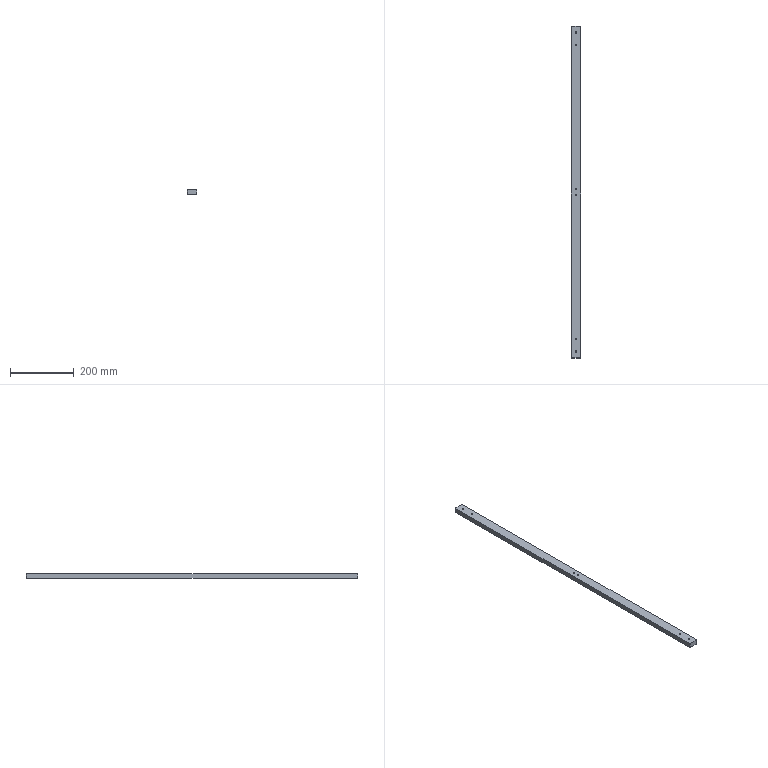Part | SolidWorks | features BaseBody 1 | 1 solid | 22 faces | box 30 x 1038 x 15 mm | volume 465386 mm3 | cylinder 12 | plane 10 | commonest cylinder face diameters 5 x8 4.2 x4
STEP:
#1=CARTESIAN_POINT('',(-2.1,529.,-7.5));
#2=VERTEX_POINT('',#1);
#3=CARTESIAN_POINT('',(2.1,529.,-7.5));
#4=VERTEX_POINT('',#3);
#5=CARTESIAN_POINT('',(0.,529.,-7.5));
#6=DIRECTION('',(0.,0.,1.));
#7=DIRECTION('',(1.,0.,0.));
#8=AXIS2_PLACEMENT_3D('',#5,#6,#7);
#9=CIRCLE('',#8,2.1);
#10=EDGE_CURVE('',#2,#4,#9,.T.);
#11=ORIENTED_EDGE('',*,*,#10,.F.);
#12=CARTESIAN_POINT('',(-2.1,529.,7.5));
#13=VERTEX_POINT('',#12);
#14=CARTESIAN_POINT('',(-2.1,529.,7.5));
#15=DIRECTION('',(0.,0.,1.));
#16=VECTOR('',#15,1000.);
#17=LINE('',#14,#16);
#18=EDGE_CURVE('',#2,#13,#17,.T.);
#19=ORIENTED_EDGE('',*,*,#18,.T.);
#20=CARTESIAN_POINT('',(2.1,529.,7.5));
#21=VERTEX_POINT('',#20);
#22=CARTESIAN_POINT('',(0.,529.,7.5));
#23=DIRECTION('',(0.,0.,1.));
#24=DIRECTION('',(1.,0.,0.));
#25=AXIS2_PLACEMENT_3D('',#22,#23,#24);
#26=CIRCLE('',#25,2.1);
#27=EDGE_CURVE('',#13,#21,#26,.T.);
#28=ORIENTED_EDGE('',*,*,#27,.T.);
#29=CARTESIAN_POINT('',(2.1,529.,7.5));
#30=DIRECTION('',(0.,0.,1.));
#31=VECTOR('',#30,1000.);
#32=LINE('',#29,#31);
#33=EDGE_CURVE('',#4,#21,#32,.T.);
#34=ORIENTED_EDGE('',*,*,#33,.F.);
#35=EDGE_LOOP('',(#11,#19,#28,#34));
#36=FACE_OUTER_BOUND('',#35,.T.);
#37=CARTESIAN_POINT('',(0.,529.,7.5));
#38=DIRECTION('',(0.,0.,1.));
#39=DIRECTION('',(1.,0.,0.));
#40=AXIS2_PLACEMENT_3D('',#37,#38,#39);
#41=CYLINDRICAL_SURFACE('',#40,2.1);
#42=ADVANCED_FACE('',(#36),#41,.F.);
#43=CARTESIAN_POINT('',(-2.1,509.,-7.5));
#44=VERTEX_POINT('',#43);
#45=CARTESIAN_POINT('',(2.1,509.,-7.5));
#46=VERTEX_POINT('',#45);
#47=CARTESIAN_POINT('',(0.,509.,-7.5));
#48=DIRECTION('',(0.,0.,1.));
#49=DIRECTION('',(1.,0.,0.));
#50=AXIS2_PLACEMENT_3D('',#47,#48,#49);
#51=CIRCLE('',#50,2.1);
#52=EDGE_CURVE('',#44,#46,#51,.T.);
#53=ORIENTED_EDGE('',*,*,#52,.F.);
#54=CARTESIAN_POINT('',(-2.1,509.,7.5));
#55=VERTEX_POINT('',#54);
#56=CARTESIAN_POINT('',(-2.1,509.,7.5));
#57=DIRECTION('',(0.,0.,1.));
#58=VECTOR('',#57,1000.);
#59=LINE('',#56,#58);
#60=EDGE_CURVE('',#44,#55,#59,.T.);
#61=ORIENTED_EDGE('',*,*,#60,.T.);
#62=CARTESIAN_POINT('',(2.1,509.,7.5));
#63=VERTEX_POINT('',#62);
#64=CARTESIAN_POINT('',(0.,509.,7.5));
#65=DIRECTION('',(0.,0.,1.));
#66=DIRECTION('',(1.,0.,0.));
#67=AXIS2_PLACEMENT_3D('',#64,#65,#66);
#68=CIRCLE('',#67,2.1);
#69=EDGE_CURVE('',#55,#63,#68,.T.);
#70=ORIENTED_EDGE('',*,*,#69,.T.);
#71=CARTESIAN_POINT('',(2.1,509.,7.5));
#72=DIRECTION('',(0.,0.,1.));
#73=VECTOR('',#72,1000.);
#74=LINE('',#71,#73);
#75=EDGE_CURVE('',#46,#63,#74,.T.);
#76=ORIENTED_EDGE('',*,*,#75,.F.);
#77=EDGE_LOOP('',(#53,#61,#70,#76));
#78=FACE_OUTER_BOUND('',#77,.T.);
#79=CARTESIAN_POINT('',(0.,509.,7.5));
#80=DIRECTION('',(0.,0.,1.));
#81=DIRECTION('',(1.,0.,0.));
#82=AXIS2_PLACEMENT_3D('',#79,#80,#81);
#83=CYLINDRICAL_SURFACE('',#82,2.1);
#84=ADVANCED_FACE('',(#78),#83,.F.);
#85=CARTESIAN_POINT('',(-2.5,1018.,-7.5));
#86=VERTEX_POINT('',#85);
#87=CARTESIAN_POINT('',(2.5,1018.,-7.5));
#88=VERTEX_POINT('',#87);
#89=CARTESIAN_POINT('',(0.,1018.,-7.5));
#90=DIRECTION('',(0.,0.,1.));
#91=DIRECTION('',(1.,0.,0.));
#92=AXIS2_PLACEMENT_3D('',#89,#90,#91);
#93=CIRCLE('',#92,2.5);
#94=EDGE_CURVE('',#86,#88,#93,.T.);
#95=ORIENTED_EDGE('',*,*,#94,.F.);
#96=CARTESIAN_POINT('',(-2.5,1018.,7.5));
#97=VERTEX_POINT('',#96);
#98=CARTESIAN_POINT('',(-2.5,1018.,7.5));
#99=DIRECTION('',(0.,0.,1.));
#100=VECTOR('',#99,1000.);
#101=LINE('',#98,#100);
#102=EDGE_CURVE('',#86,#97,#101,.T.);
#103=ORIENTED_EDGE('',*,*,#102,.T.);
#104=CARTESIAN_POINT('',(2.5,1018.,7.5));
#105=VERTEX_POINT('',#104);
#106=CARTESIAN_POINT('',(0.,1018.,7.5));
#107=DIRECTION('',(0.,0.,1.));
#108=DIRECTION('',(1.,0.,0.));
#109=AXIS2_PLACEMENT_3D('',#106,#107,#108);
#110=CIRCLE('',#109,2.5);
#111=EDGE_CURVE('',#97,#105,#110,.T.);
#112=ORIENTED_EDGE('',*,*,#111,.T.);
#113=CARTESIAN_POINT('',(2.5,1018.,7.5));
#114=DIRECTION('',(0.,0.,1.));
#115=VECTOR('',#114,1000.);
#116=LINE('',#113,#115);
#117=EDGE_CURVE('',#88,#105,#116,.T.);
#118=ORIENTED_EDGE('',*,*,#117,.F.);
#119=EDGE_LOOP('',(#95,#103,#112,#118));
#120=FACE_OUTER_BOUND('',#119,.T.);
#121=CARTESIAN_POINT('',(0.,1018.,7.5));
#122=DIRECTION('',(0.,0.,1.));
#123=DIRECTION('',(1.,0.,0.));
#124=AXIS2_PLACEMENT_3D('',#121,#122,#123);
#125=CYLINDRICAL_SURFACE('',#124,2.5);
#126=ADVANCED_FACE('',(#120),#125,.F.);
#127=CARTESIAN_POINT('',(-2.5,978.,-7.5));
#128=VERTEX_POINT('',#127);
#129=CARTESIAN_POINT('',(2.5,978.,-7.5));
#130=VERTEX_POINT('',#129);
#131=CARTESIAN_POINT('',(0.,978.,-7.5));
#132=DIRECTION('',(0.,0.,1.));
#133=DIRECTION('',(1.,0.,0.));
#134=AXIS2_PLACEMENT_3D('',#131,#132,#133);
#135=CIRCLE('',#134,2.5);
#136=EDGE_CURVE('',#128,#130,#135,.T.);
#137=ORIENTED_EDGE('',*,*,#136,.F.);
#138=CARTESIAN_POINT('',(-2.5,978.,7.5));
#139=VERTEX_POINT('',#138);
#140=CARTESIAN_POINT('',(-2.5,978.,7.5));
#141=DIRECTION('',(0.,0.,1.));
#142=VECTOR('',#141,1000.);
#143=LINE('',#140,#142);
#144=EDGE_CURVE('',#128,#139,#143,.T.);
#145=ORIENTED_EDGE('',*,*,#144,.T.);
#146=CARTESIAN_POINT('',(2.5,978.,7.5));
#147=VERTEX_POINT('',#146);
#148=CARTESIAN_POINT('',(0.,978.,7.5));
#149=DIRECTION('',(0.,0.,1.));
#150=DIRECTION('',(1.,0.,0.));
#151=AXIS2_PLACEMENT_3D('',#148,#149,#150);
#152=CIRCLE('',#151,2.5);
#153=EDGE_CURVE('',#139,#147,#152,.T.);
#154=ORIENTED_EDGE('',*,*,#153,.T.);
#155=CARTESIAN_POINT('',(2.5,978.,7.5));
#156=DIRECTION('',(0.,0.,1.));
#157=VECTOR('',#156,1000.);
#158=LINE('',#155,#157);
#159=EDGE_CURVE('',#130,#147,#158,.T.);
#160=ORIENTED_EDGE('',*,*,#159,.F.);
#161=EDGE_LOOP('',(#137,#145,#154,#160));
#162=FACE_OUTER_BOUND('',#161,.T.);
#163=CARTESIAN_POINT('',(0.,978.,7.5));
#164=DIRECTION('',(0.,0.,1.));
#165=DIRECTION('',(1.,0.,0.));
#166=AXIS2_PLACEMENT_3D('',#163,#164,#165);
#167=CYLINDRICAL_SURFACE('',#166,2.5);
#168=ADVANCED_FACE('',(#162),#167,.F.);
#169=CARTESIAN_POINT('',(-2.5,20.,-7.5));
#170=VERTEX_POINT('',#169);
#171=CARTESIAN_POINT('',(2.5,20.,-7.5));
#172=VERTEX_POINT('',#171);
#173=CARTESIAN_POINT('',(0.,20.,-7.5));
#174=DIRECTION('',(0.,0.,1.));
#175=DIRECTION('',(1.,0.,0.));
#176=AXIS2_PLACEMENT_3D('',#173,#174,#175);
#177=CIRCLE('',#176,2.5);
#178=EDGE_CURVE('',#170,#172,#177,.T.);
#179=ORIENTED_EDGE('',*,*,#178,.F.);
#180=CARTESIAN_POINT('',(-2.5,20.,7.5));
#181=VERTEX_POINT('',#180);
#182=CARTESIAN_POINT('',(-2.5,20.,7.5));
#183=DIRECTION('',(0.,0.,1.));
#184=VECTOR('',#183,1000.);
#185=LINE('',#182,#184);
#186=EDGE_CURVE('',#170,#181,#185,.T.);
#187=ORIENTED_EDGE('',*,*,#186,.T.);
#188=CARTESIAN_POINT('',(2.5,20.,7.5));
#189=VERTEX_POINT('',#188);
#190=CARTESIAN_POINT('',(0.,20.,7.5));
#191=DIRECTION('',(0.,0.,1.));
#192=DIRECTION('',(1.,0.,0.));
#193=AXIS2_PLACEMENT_3D('',#190,#191,#192);
#194=CIRCLE('',#193,2.5);
#195=EDGE_CURVE('',#181,#189,#194,.T.);
#196=ORIENTED_EDGE('',*,*,#195,.T.);
#197=CARTESIAN_POINT('',(2.5,20.,7.5));
#198=DIRECTION('',(0.,0.,1.));
#199=VECTOR('',#198,1000.);
#200=LINE('',#197,#199);
#201=EDGE_CURVE('',#172,#189,#200,.T.);
#202=ORIENTED_EDGE('',*,*,#201,.F.);
#203=EDGE_LOOP('',(#179,#187,#196,#202));
#204=FACE_OUTER_BOUND('',#203,.T.);
#205=CARTESIAN_POINT('',(0.,20.,7.5));
#206=DIRECTION('',(0.,0.,1.));
#207=DIRECTION('',(1.,0.,0.));
#208=AXIS2_PLACEMENT_3D('',#205,#206,#207);
#209=CYLINDRICAL_SURFACE('',#208,2.5);
#210=ADVANCED_FACE('',(#204),#209,.F.);
#211=CARTESIAN_POINT('',(-2.5,60.,-7.5));
#212=VERTEX_POINT('',#211);
#213=CARTESIAN_POINT('',(2.5,60.,-7.5));
#214=VERTEX_POINT('',#213);
#215=CARTESIAN_POINT('',(0.,60.,-7.5));
#216=DIRECTION('',(0.,0.,1.));
#217=DIRECTION('',(1.,0.,0.));
#218=AXIS2_PLACEMENT_3D('',#215,#216,#217);
#219=CIRCLE('',#218,2.5);
#220=EDGE_CURVE('',#212,#214,#219,.T.);
#221=ORIENTED_EDGE('',*,*,#220,.F.);
#222=CARTESIAN_POINT('',(-2.5,60.,7.5));
#223=VERTEX_POINT('',#222);
#224=CARTESIAN_POINT('',(-2.5,60.,7.5));
#225=DIRECTION('',(0.,0.,1.));
#226=VECTOR('',#225,1000.);
#227=LINE('',#224,#226);
#228=EDGE_CURVE('',#212,#223,#227,.T.);
#229=ORIENTED_EDGE('',*,*,#228,.T.);
#230=CARTESIAN_POINT('',(2.5,60.,7.5));
#231=VERTEX_POINT('',#230);
#232=CARTESIAN_POINT('',(0.,60.,7.5));
#233=DIRECTION('',(0.,0.,1.));
#234=DIRECTION('',(1.,0.,0.));
#235=AXIS2_PLACEMENT_3D('',#232,#233,#234);
#236=CIRCLE('',#235,2.5);
#237=EDGE_CURVE('',#223,#231,#236,.T.);
#238=ORIENTED_EDGE('',*,*,#237,.T.);
#239=CARTESIAN_POINT('',(2.5,60.,7.5));
#240=DIRECTION('',(0.,0.,1.));
#241=VECTOR('',#240,1000.);
#242=LINE('',#239,#241);
#243=EDGE_CURVE('',#214,#231,#242,.T.);
#244=ORIENTED_EDGE('',*,*,#243,.F.);
#245=EDGE_LOOP('',(#221,#229,#238,#244));
#246=FACE_OUTER_BOUND('',#245,.T.);
#247=CARTESIAN_POINT('',(0.,60.,7.5));
#248=DIRECTION('',(0.,0.,1.));
#249=DIRECTION('',(1.,0.,0.));
#250=AXIS2_PLACEMENT_3D('',#247,#248,#249);
#251=CYLINDRICAL_SURFACE('',#250,2.5);
#252=ADVANCED_FACE('',(#246),#251,.F.);
#253=CARTESIAN_POINT('',(-15.,1036.,-7.5));
#254=VERTEX_POINT('',#253);
#255=CARTESIAN_POINT('',(-13.,1038.,-7.5));
#256=VERTEX_POINT('',#255);
#257=CARTESIAN_POINT('',(-13.,1038.,-7.5));
#258=DIRECTION('',(0.7071,0.7071,0.));
#259=VECTOR('',#258,1000.);
#260=LINE('',#257,#259);
#261=EDGE_CURVE('',#254,#256,#260,.T.);
#262=ORIENTED_EDGE('',*,*,#261,.F.);
#263=CARTESIAN_POINT('',(-15.,1036.,7.5));
#264=VERTEX_POINT('',#263);
#265=CARTESIAN_POINT('',(-15.,1036.,-7.5));
#266=DIRECTION('',(0.,0.,-1.));
#267=VECTOR('',#266,1000.);
#268=LINE('',#265,#267);
#269=EDGE_CURVE('',#264,#254,#268,.T.);
#270=ORIENTED_EDGE('',*,*,#269,.F.);
#271=CARTESIAN_POINT('',(-13.,1038.,7.5));
#272=VERTEX_POINT('',#271);
#273=CARTESIAN_POINT('',(-13.,1038.,7.5));
#274=DIRECTION('',(-0.7071,-0.7071,0.));
#275=VECTOR('',#274,1000.);
#276=LINE('',#273,#275);
#277=EDGE_CURVE('',#272,#264,#276,.T.);
#278=ORIENTED_EDGE('',*,*,#277,.F.);
#279=CARTESIAN_POINT('',(-13.,1038.,7.5));
#280=DIRECTION('',(0.,0.,1.));
#281=VECTOR('',#280,1000.);
#282=LINE('',#279,#281);
#283=EDGE_CURVE('',#256,#272,#282,.T.);
#284=ORIENTED_EDGE('',*,*,#283,.F.);
#285=EDGE_LOOP('',(#262,#270,#278,#284));
#286=FACE_OUTER_BOUND('',#285,.T.);
#287=CARTESIAN_POINT('',(-13.,1038.,0.));
#288=DIRECTION('',(-0.7071,0.7071,0.));
#289=DIRECTION('',(0.,0.,1.));
#290=AXIS2_PLACEMENT_3D('',#287,#288,#289);
#291=PLANE('',#290);
#292=ADVANCED_FACE('',(#286),#291,.T.);
#293=CARTESIAN_POINT('',(15.,1036.,7.5));
#294=VERTEX_POINT('',#293);
#295=CARTESIAN_POINT('',(13.,1038.,7.5));
#296=VERTEX_POINT('',#295);
#297=CARTESIAN_POINT('',(13.,1038.,7.5));
#298=DIRECTION('',(-0.7071,0.7071,0.));
#299=VECTOR('',#298,1000.);
#300=LINE('',#297,#299);
#301=EDGE_CURVE('',#294,#296,#300,.T.);
#302=ORIENTED_EDGE('',*,*,#301,.F.);
#303=CARTESIAN_POINT('',(15.,1036.,-7.5));
#304=VERTEX_POINT('',#303);
#305=CARTESIAN_POINT('',(15.,1036.,7.5));
#306=DIRECTION('',(0.,0.,1.));
#307=VECTOR('',#306,1000.);
#308=LINE('',#305,#307);
#309=EDGE_CURVE('',#304,#294,#308,.T.);
#310=ORIENTED_EDGE('',*,*,#309,.F.);
#311=CARTESIAN_POINT('',(13.,1038.,-7.5));
#312=VERTEX_POINT('',#311);
#313=CARTESIAN_POINT('',(13.,1038.,-7.5));
#314=DIRECTION('',(0.7071,-0.7071,0.));
#315=VECTOR('',#314,1000.);
#316=LINE('',#313,#315);
#317=EDGE_CURVE('',#312,#304,#316,.T.);
#318=ORIENTED_EDGE('',*,*,#317,.F.);
#319=CARTESIAN_POINT('',(13.,1038.,-7.5));
#320=DIRECTION('',(0.,0.,-1.));
#321=VECTOR('',#320,1000.);
#322=LINE('',#319,#321);
#323=EDGE_CURVE('',#296,#312,#322,.T.);
#324=ORIENTED_EDGE('',*,*,#323,.F.);
#325=EDGE_LOOP('',(#302,#310,#318,#324));
#326=FACE_OUTER_BOUND('',#325,.T.);
#327=CARTESIAN_POINT('',(13.,1038.,0.));
#328=DIRECTION('',(0.7071,0.7071,0.));
#329=DIRECTION('',(0.,0.,-1.));
#330=AXIS2_PLACEMENT_3D('',#327,#328,#329);
#331=PLANE('',#330);
#332=ADVANCED_FACE('',(#326),#331,.T.);
#333=CARTESIAN_POINT('',(-13.,0.,-7.5));
#334=VERTEX_POINT('',#333);
#335=CARTESIAN_POINT('',(-15.,2.,-7.5));
#336=VERTEX_POINT('',#335);
#337=CARTESIAN_POINT('',(-15.,2.,-7.5));
#338=DIRECTION('',(-0.7071,0.7071,0.));
#339=VECTOR('',#338,1000.);
#340=LINE('',#337,#339);
#341=EDGE_CURVE('',#334,#336,#340,.T.);
#342=ORIENTED_EDGE('',*,*,#341,.F.);
#343=CARTESIAN_POINT('',(-13.,0.,7.5));
#344=VERTEX_POINT('',#343);
#345=CARTESIAN_POINT('',(-13.,0.,0.));
#346=DIRECTION('',(0.,0.,-1.));
#347=VECTOR('',#346,1000.);
#348=LINE('',#345,#347);
#349=EDGE_CURVE('',#344,#334,#348,.T.);
#350=ORIENTED_EDGE('',*,*,#349,.F.);
#351=CARTESIAN_POINT('',(-15.,2.,7.5));
#352=VERTEX_POINT('',#351);
#353=CARTESIAN_POINT('',(-15.,2.,7.5));
#354=DIRECTION('',(0.7071,-0.7071,0.));
#355=VECTOR('',#354,1000.);
#356=LINE('',#353,#355);
#357=EDGE_CURVE('',#352,#344,#356,.T.);
#358=ORIENTED_EDGE('',*,*,#357,.F.);
#359=CARTESIAN_POINT('',(-15.,2.,-7.5));
#360=DIRECTION('',(0.,0.,1.));
#361=VECTOR('',#360,1000.);
#362=LINE('',#359,#361);
#363=EDGE_CURVE('',#336,#352,#362,.T.);
#364=ORIENTED_EDGE('',*,*,#363,.F.);
#365=EDGE_LOOP('',(#342,#350,#358,#364));
#366=FACE_OUTER_BOUND('',#365,.T.);
#367=CARTESIAN_POINT('',(-15.,2.,-7.5));
#368=DIRECTION('',(0.7071,0.7071,0.));
#369=DIRECTION('',(0.,0.,-1.));
#370=AXIS2_PLACEMENT_3D('',#367,#368,#369);
#371=PLANE('',#370);
#372=ADVANCED_FACE('',(#366),#371,.F.);
#373=CARTESIAN_POINT('',(13.,0.,7.5));
#374=VERTEX_POINT('',#373);
#375=CARTESIAN_POINT('',(15.,2.,7.5));
#376=VERTEX_POINT('',#375);
#377=CARTESIAN_POINT('',(15.,2.,7.5));
#378=DIRECTION('',(0.7071,0.7071,0.));
#379=VECTOR('',#378,1000.);
#380=LINE('',#377,#379);
#381=EDGE_CURVE('',#374,#376,#380,.T.);
#382=ORIENTED_EDGE('',*,*,#381,.F.);
#383=CARTESIAN_POINT('',(13.,0.,-7.5));
#384=VERTEX_POINT('',#383);
#385=CARTESIAN_POINT('',(13.,0.,0.));
#386=DIRECTION('',(0.,0.,1.));
#387=VECTOR('',#386,1000.);
#388=LINE('',#385,#387);
#389=EDGE_CURVE('',#384,#374,#388,.T.);
#390=ORIENTED_EDGE('',*,*,#389,.F.);
#391=CARTESIAN_POINT('',(15.,2.,-7.5));
#392=VERTEX_POINT('',#391);
#393=CARTESIAN_POINT('',(15.,2.,-7.5));
#394=DIRECTION('',(-0.7071,-0.7071,0.));
#395=VECTOR('',#394,1000.);
#396=LINE('',#393,#395);
#397=EDGE_CURVE('',#392,#384,#396,.T.);
#398=ORIENTED_EDGE('',*,*,#397,.F.);
#399=CARTESIAN_POINT('',(15.,2.,-7.5));
#400=DIRECTION('',(0.,0.,-1.));
#401=VECTOR('',#400,1000.);
#402=LINE('',#399,#401);
#403=EDGE_CURVE('',#376,#392,#402,.T.);
#404=ORIENTED_EDGE('',*,*,#403,.F.);
#405=EDGE_LOOP('',(#382,#390,#398,#404));
#406=FACE_OUTER_BOUND('',#405,.T.);
#407=CARTESIAN_POINT('',(15.,2.,-7.5));
#408=DIRECTION('',(-0.7071,0.7071,0.));
#409=DIRECTION('',(0.,0.,1.));
#410=AXIS2_PLACEMENT_3D('',#407,#408,#409);
#411=PLANE('',#410);
#412=ADVANCED_FACE('',(#406),#411,.F.);
#413=CARTESIAN_POINT('',(-15.,0.,-7.5));
#414=DIRECTION('',(-1.,0.,0.));
#415=VECTOR('',#414,1000.);
#416=LINE('',#413,#415);
#417=EDGE_CURVE('',#384,#334,#416,.T.);
#418=ORIENTED_EDGE('',*,*,#417,.F.);
#419=ORIENTED_EDGE('',*,*,#389,.T.);
#420=CARTESIAN_POINT('',(-15.,0.,7.5));
#421=DIRECTION('',(1.,0.,0.));
#422=VECTOR('',#421,1000.);
#423=LINE('',#420,#422);
#424=EDGE_CURVE('',#344,#374,#423,.T.);
#425=ORIENTED_EDGE('',*,*,#424,.F.);
#426=ORIENTED_EDGE('',*,*,#349,.T.);
#427=EDGE_LOOP('',(#418,#419,#425,#426));
#428=FACE_OUTER_BOUND('',#427,.T.);
#429=CARTESIAN_POINT('',(0.,0.,0.));
#430=DIRECTION('',(0.,1.,0.));
#431=DIRECTION('',(1.,0.,0.));
#432=AXIS2_PLACEMENT_3D('',#429,#430,#431);
#433=PLANE('',#432);
#434=ADVANCED_FACE('',(#428),#433,.F.);
#435=CARTESIAN_POINT('',(-15.,1038.,7.5));
#436=DIRECTION('',(1.,0.,0.));
#437=VECTOR('',#436,1000.);
#438=LINE('',#435,#437);
#439=EDGE_CURVE('',#272,#296,#438,.T.);
#440=ORIENTED_EDGE('',*,*,#439,.T.);
#441=ORIENTED_EDGE('',*,*,#323,.T.);
#442=CARTESIAN_POINT('',(-15.,1038.,-7.5));
#443=DIRECTION('',(-1.,0.,0.));
#444=VECTOR('',#443,1000.);
#445=LINE('',#442,#444);
#446=EDGE_CURVE('',#312,#256,#445,.T.);
#447=ORIENTED_EDGE('',*,*,#446,.T.);
#448=ORIENTED_EDGE('',*,*,#283,.T.);
#449=EDGE_LOOP('',(#440,#441,#447,#448));
#450=FACE_OUTER_BOUND('',#449,.T.);
#451=CARTESIAN_POINT('',(0.,1038.,0.));
#452=DIRECTION('',(0.,1.,0.));
#453=DIRECTION('',(1.,0.,0.));
#454=AXIS2_PLACEMENT_3D('',#451,#452,#453);
#455=PLANE('',#454);
#456=ADVANCED_FACE('',(#450),#455,.T.);
#457=CARTESIAN_POINT('',(0.,60.,7.5));
#458=DIRECTION('',(0.,0.,1.));
#459=DIRECTION('',(1.,0.,0.));
#460=AXIS2_PLACEMENT_3D('',#457,#458,#459);
#461=CIRCLE('',#460,2.5);
#462=EDGE_CURVE('',#231,#223,#461,.T.);
#463=ORIENTED_EDGE('',*,*,#462,.F.);
#464=ORIENTED_EDGE('',*,*,#237,.F.);
#465=EDGE_LOOP('',(#463,#464));
#466=FACE_BOUND('',#465,.T.);
#467=CARTESIAN_POINT('',(0.,20.,7.5));
#468=DIRECTION('',(0.,0.,1.));
#469=DIRECTION('',(1.,0.,0.));
#470=AXIS2_PLACEMENT_3D('',#467,#468,#469);
#471=CIRCLE('',#470,2.5);
#472=EDGE_CURVE('',#189,#181,#471,.T.);
#473=ORIENTED_EDGE('',*,*,#472,.F.);
#474=ORIENTED_EDGE('',*,*,#195,.F.);
#475=EDGE_LOOP('',(#473,#474));
#476=FACE_BOUND('',#475,.T.);
#477=CARTESIAN_POINT('',(0.,978.,7.5));
#478=DIRECTION('',(0.,0.,1.));
#479=DIRECTION('',(1.,0.,0.));
#480=AXIS2_PLACEMENT_3D('',#477,#478,#479);
#481=CIRCLE('',#480,2.5);
#482=EDGE_CURVE('',#147,#139,#481,.T.);
#483=ORIENTED_EDGE('',*,*,#482,.F.);
#484=ORIENTED_EDGE('',*,*,#153,.F.);
#485=EDGE_LOOP('',(#483,#484));
#486=FACE_BOUND('',#485,.T.);
#487=CARTESIAN_POINT('',(0.,1018.,7.5));
#488=DIRECTION('',(0.,0.,1.));
#489=DIRECTION('',(1.,0.,0.));
#490=AXIS2_PLACEMENT_3D('',#487,#488,#489);
#491=CIRCLE('',#490,2.5);
#492=EDGE_CURVE('',#105,#97,#491,.T.);
#493=ORIENTED_EDGE('',*,*,#492,.F.);
#494=ORIENTED_EDGE('',*,*,#111,.F.);
#495=EDGE_LOOP('',(#493,#494));
#496=FACE_BOUND('',#495,.T.);
#497=CARTESIAN_POINT('',(0.,509.,7.5));
#498=DIRECTION('',(0.,0.,1.));
#499=DIRECTION('',(1.,0.,0.));
#500=AXIS2_PLACEMENT_3D('',#497,#498,#499);
#501=CIRCLE('',#500,2.1);
#502=EDGE_CURVE('',#63,#55,#501,.T.);
#503=ORIENTED_EDGE('',*,*,#502,.F.);
#504=ORIENTED_EDGE('',*,*,#69,.F.);
#505=EDGE_LOOP('',(#503,#504));
#506=FACE_BOUND('',#505,.T.);
#507=CARTESIAN_POINT('',(0.,529.,7.5));
#508=DIRECTION('',(0.,0.,1.));
#509=DIRECTION('',(1.,0.,0.));
#510=AXIS2_PLACEMENT_3D('',#507,#508,#509);
#511=CIRCLE('',#510,2.1);
#512=EDGE_CURVE('',#21,#13,#511,.T.);
#513=ORIENTED_EDGE('',*,*,#512,.F.);
#514=ORIENTED_EDGE('',*,*,#27,.F.);
#515=EDGE_LOOP('',(#513,#514));
#516=FACE_BOUND('',#515,.T.);
#517=ORIENTED_EDGE('',*,*,#424,.T.);
#518=ORIENTED_EDGE('',*,*,#381,.T.);
#519=CARTESIAN_POINT('',(15.,1038.,7.5));
#520=DIRECTION('',(0.,-1.,0.));
#521=VECTOR('',#520,1000.);
#522=LINE('',#519,#521);
#523=EDGE_CURVE('',#294,#376,#522,.T.);
#524=ORIENTED_EDGE('',*,*,#523,.F.);
#525=ORIENTED_EDGE('',*,*,#301,.T.);
#526=ORIENTED_EDGE('',*,*,#439,.F.);
#527=ORIENTED_EDGE('',*,*,#277,.T.);
#528=CARTESIAN_POINT('',(-15.,1038.,7.5));
#529=DIRECTION('',(0.,-1.,0.));
#530=VECTOR('',#529,1000.);
#531=LINE('',#528,#530);
#532=EDGE_CURVE('',#264,#352,#531,.T.);
#533=ORIENTED_EDGE('',*,*,#532,.T.);
#534=ORIENTED_EDGE('',*,*,#357,.T.);
#535=EDGE_LOOP('',(#517,#518,#524,#525,#526,#527,#533,#534));
#536=FACE_OUTER_BOUND('',#535,.T.);
#537=CARTESIAN_POINT('',(-15.,1038.,7.5));
#538=DIRECTION('',(0.,0.,-1.));
#539=DIRECTION('',(0.,-1.,0.));
#540=AXIS2_PLACEMENT_3D('',#537,#538,#539);
#541=PLANE('',#540);
#542=ADVANCED_FACE('',(#466,#476,#486,#496,#506,#516,#536),#541,.F.);
#543=CARTESIAN_POINT('',(-15.,1038.,-7.5));
#544=DIRECTION('',(0.,-1.,0.));
#545=VECTOR('',#544,1000.);
#546=LINE('',#543,#545);
#547=EDGE_CURVE('',#254,#336,#546,.T.);
#548=ORIENTED_EDGE('',*,*,#547,.T.);
#549=ORIENTED_EDGE('',*,*,#363,.T.);
#550=ORIENTED_EDGE('',*,*,#532,.F.);
#551=ORIENTED_EDGE('',*,*,#269,.T.);
#552=EDGE_LOOP('',(#548,#549,#550,#551));
#553=FACE_OUTER_BOUND('',#552,.T.);
#554=CARTESIAN_POINT('',(-15.,1038.,-7.5));
#555=DIRECTION('',(1.,0.,0.));
#556=DIRECTION('',(0.,0.,-1.));
#557=AXIS2_PLACEMENT_3D('',#554,#555,#556);
#558=PLANE('',#557);
#559=ADVANCED_FACE('',(#553),#558,.F.);
#560=CARTESIAN_POINT('',(0.,60.,-7.5));
#561=DIRECTION('',(0.,0.,1.));
#562=DIRECTION('',(1.,0.,0.));
#563=AXIS2_PLACEMENT_3D('',#560,#561,#562);
#564=CIRCLE('',#563,2.5);
#565=EDGE_CURVE('',#214,#212,#564,.T.);
#566=ORIENTED_EDGE('',*,*,#565,.T.);
#567=ORIENTED_EDGE('',*,*,#220,.T.);
#568=EDGE_LOOP('',(#566,#567));
#569=FACE_BOUND('',#568,.T.);
#570=CARTESIAN_POINT('',(0.,20.,-7.5));
#571=DIRECTION('',(0.,0.,1.));
#572=DIRECTION('',(1.,0.,0.));
#573=AXIS2_PLACEMENT_3D('',#570,#571,#572);
#574=CIRCLE('',#573,2.5);
#575=EDGE_CURVE('',#172,#170,#574,.T.);
#576=ORIENTED_EDGE('',*,*,#575,.T.);
#577=ORIENTED_EDGE('',*,*,#178,.T.);
#578=EDGE_LOOP('',(#576,#577));
#579=FACE_BOUND('',#578,.T.);
#580=CARTESIAN_POINT('',(0.,978.,-7.5));
#581=DIRECTION('',(0.,0.,1.));
#582=DIRECTION('',(1.,0.,0.));
#583=AXIS2_PLACEMENT_3D('',#580,#581,#582);
#584=CIRCLE('',#583,2.5);
#585=EDGE_CURVE('',#130,#128,#584,.T.);
#586=ORIENTED_EDGE('',*,*,#585,.T.);
#587=ORIENTED_EDGE('',*,*,#136,.T.);
#588=EDGE_LOOP('',(#586,#587));
#589=FACE_BOUND('',#588,.T.);
#590=CARTESIAN_POINT('',(0.,1018.,-7.5));
#591=DIRECTION('',(0.,0.,1.));
#592=DIRECTION('',(1.,0.,0.));
#593=AXIS2_PLACEMENT_3D('',#590,#591,#592);
#594=CIRCLE('',#593,2.5);
#595=EDGE_CURVE('',#88,#86,#594,.T.);
#596=ORIENTED_EDGE('',*,*,#595,.T.);
#597=ORIENTED_EDGE('',*,*,#94,.T.);
#598=EDGE_LOOP('',(#596,#597));
#599=FACE_BOUND('',#598,.T.);
#600=CARTESIAN_POINT('',(0.,509.,-7.5));
#601=DIRECTION('',(0.,0.,1.));
#602=DIRECTION('',(1.,0.,0.));
#603=AXIS2_PLACEMENT_3D('',#600,#601,#602);
#604=CIRCLE('',#603,2.1);
#605=EDGE_CURVE('',#46,#44,#604,.T.);
#606=ORIENTED_EDGE('',*,*,#605,.T.);
#607=ORIENTED_EDGE('',*,*,#52,.T.);
#608=EDGE_LOOP('',(#606,#607));
#609=FACE_BOUND('',#608,.T.);
#610=CARTESIAN_POINT('',(0.,529.,-7.5));
#611=DIRECTION('',(0.,0.,1.));
#612=DIRECTION('',(1.,0.,0.));
#613=AXIS2_PLACEMENT_3D('',#610,#611,#612);
#614=CIRCLE('',#613,2.1);
#615=EDGE_CURVE('',#4,#2,#614,.T.);
#616=ORIENTED_EDGE('',*,*,#615,.T.);
#617=ORIENTED_EDGE('',*,*,#10,.T.);
#618=EDGE_LOOP('',(#616,#617));
#619=FACE_BOUND('',#618,.T.);
#620=CARTESIAN_POINT('',(15.,1038.,-7.5));
#621=DIRECTION('',(0.,-1.,0.));
#622=VECTOR('',#621,1000.);
#623=LINE('',#620,#622);
#624=EDGE_CURVE('',#304,#392,#623,.T.);
#625=ORIENTED_EDGE('',*,*,#624,.T.);
#626=ORIENTED_EDGE('',*,*,#397,.T.);
#627=ORIENTED_EDGE('',*,*,#417,.T.);
#628=ORIENTED_EDGE('',*,*,#341,.T.);
#629=ORIENTED_EDGE('',*,*,#547,.F.);
#630=ORIENTED_EDGE('',*,*,#261,.T.);
#631=ORIENTED_EDGE('',*,*,#446,.F.);
#632=ORIENTED_EDGE('',*,*,#317,.T.);
#633=EDGE_LOOP('',(#625,#626,#627,#628,#629,#630,#631,#632));
#634=FACE_OUTER_BOUND('',#633,.T.);
#635=CARTESIAN_POINT('',(-15.,1038.,-7.5));
#636=DIRECTION('',(0.,0.,1.));
#637=DIRECTION('',(1.,0.,0.));
#638=AXIS2_PLACEMENT_3D('',#635,#636,#637);
#639=PLANE('',#638);
#640=ADVANCED_FACE('',(#569,#579,#589,#599,#609,#619,#634),#639,.F.);
#641=ORIENTED_EDGE('',*,*,#523,.T.);
#642=ORIENTED_EDGE('',*,*,#403,.T.);
#643=ORIENTED_EDGE('',*,*,#624,.F.);
#644=ORIENTED_EDGE('',*,*,#309,.T.);
#645=EDGE_LOOP('',(#641,#642,#643,#644));
#646=FACE_OUTER_BOUND('',#645,.T.);
#647=CARTESIAN_POINT('',(15.,1038.,-7.5));
#648=DIRECTION('',(-1.,0.,0.));
#649=DIRECTION('',(0.,1.,0.));
#650=AXIS2_PLACEMENT_3D('',#647,#648,#649);
#651=PLANE('',#650);
#652=ADVANCED_FACE('',(#646),#651,.F.);
#653=ORIENTED_EDGE('',*,*,#228,.F.);
#654=ORIENTED_EDGE('',*,*,#565,.F.);
#655=ORIENTED_EDGE('',*,*,#243,.T.);
#656=ORIENTED_EDGE('',*,*,#462,.T.);
#657=EDGE_LOOP('',(#653,#654,#655,#656));
#658=FACE_OUTER_BOUND('',#657,.T.);
#659=CARTESIAN_POINT('',(0.,60.,7.5));
#660=DIRECTION('',(0.,0.,1.));
#661=DIRECTION('',(1.,0.,0.));
#662=AXIS2_PLACEMENT_3D('',#659,#660,#661);
#663=CYLINDRICAL_SURFACE('',#662,2.5);
#664=ADVANCED_FACE('',(#658),#663,.F.);
#665=ORIENTED_EDGE('',*,*,#186,.F.);
#666=ORIENTED_EDGE('',*,*,#575,.F.);
#667=ORIENTED_EDGE('',*,*,#201,.T.);
#668=ORIENTED_EDGE('',*,*,#472,.T.);
#669=EDGE_LOOP('',(#665,#666,#667,#668));
#670=FACE_OUTER_BOUND('',#669,.T.);
#671=CARTESIAN_POINT('',(0.,20.,7.5));
#672=DIRECTION('',(0.,0.,1.));
#673=DIRECTION('',(1.,0.,0.));
#674=AXIS2_PLACEMENT_3D('',#671,#672,#673);
#675=CYLINDRICAL_SURFACE('',#674,2.5);
#676=ADVANCED_FACE('',(#670),#675,.F.);
#677=ORIENTED_EDGE('',*,*,#144,.F.);
#678=ORIENTED_EDGE('',*,*,#585,.F.);
#679=ORIENTED_EDGE('',*,*,#159,.T.);
#680=ORIENTED_EDGE('',*,*,#482,.T.);
#681=EDGE_LOOP('',(#677,#678,#679,#680));
#682=FACE_OUTER_BOUND('',#681,.T.);
#683=CARTESIAN_POINT('',(0.,978.,7.5));
#684=DIRECTION('',(0.,0.,1.));
#685=DIRECTION('',(1.,0.,0.));
#686=AXIS2_PLACEMENT_3D('',#683,#684,#685);
#687=CYLINDRICAL_SURFACE('',#686,2.5);
#688=ADVANCED_FACE('',(#682),#687,.F.);
#689=ORIENTED_EDGE('',*,*,#102,.F.);
#690=ORIENTED_EDGE('',*,*,#595,.F.);
#691=ORIENTED_EDGE('',*,*,#117,.T.);
#692=ORIENTED_EDGE('',*,*,#492,.T.);
#693=EDGE_LOOP('',(#689,#690,#691,#692));
#694=FACE_OUTER_BOUND('',#693,.T.);
#695=CARTESIAN_POINT('',(0.,1018.,7.5));
#696=DIRECTION('',(0.,0.,1.));
#697=DIRECTION('',(1.,0.,0.));
#698=AXIS2_PLACEMENT_3D('',#695,#696,#697);
#699=CYLINDRICAL_SURFACE('',#698,2.5);
#700=ADVANCED_FACE('',(#694),#699,.F.);
#701=ORIENTED_EDGE('',*,*,#60,.F.);
#702=ORIENTED_EDGE('',*,*,#605,.F.);
#703=ORIENTED_EDGE('',*,*,#75,.T.);
#704=ORIENTED_EDGE('',*,*,#502,.T.);
#705=EDGE_LOOP('',(#701,#702,#703,#704));
#706=FACE_OUTER_BOUND('',#705,.T.);
#707=CARTESIAN_POINT('',(0.,509.,7.5));
#708=DIRECTION('',(0.,0.,1.));
#709=DIRECTION('',(1.,0.,0.));
#710=AXIS2_PLACEMENT_3D('',#707,#708,#709);
#711=CYLINDRICAL_SURFACE('',#710,2.1);
#712=ADVANCED_FACE('',(#706),#711,.F.);
#713=ORIENTED_EDGE('',*,*,#18,.F.);
#714=ORIENTED_EDGE('',*,*,#615,.F.);
#715=ORIENTED_EDGE('',*,*,#33,.T.);
#716=ORIENTED_EDGE('',*,*,#512,.T.);
#717=EDGE_LOOP('',(#713,#714,#715,#716));
#718=FACE_OUTER_BOUND('',#717,.T.);
#719=CARTESIAN_POINT('',(0.,529.,7.5));
#720=DIRECTION('',(0.,0.,1.));
#721=DIRECTION('',(1.,0.,0.));
#722=AXIS2_PLACEMENT_3D('',#719,#720,#721);
#723=CYLINDRICAL_SURFACE('',#722,2.1);
#724=ADVANCED_FACE('',(#718),#723,.F.);
#725=CLOSED_SHELL('',(#42,#84,#126,#168,#210,#252,#292,#332,#372,#412,#434,#456,#542,#559,#640,#652,#664,#676,#688,#700,#712,#724));
#726=MANIFOLD_SOLID_BREP('',#725);
#727=CARTESIAN_POINT('',(0.,0.,0.));
#728=DIRECTION('',(0.,0.,1.));
#729=DIRECTION('',(1.,0.,0.));
#730=AXIS2_PLACEMENT_3D('',#727,#728,#729);
#731=(LENGTH_UNIT()NAMED_UNIT(*)SI_UNIT(.MILLI.,.METRE.));
#732=UNCERTAINTY_MEASURE_WITH_UNIT(LENGTH_MEASURE(0.00001),#731,'','');
#733=(NAMED_UNIT(*)PLANE_ANGLE_UNIT()SI_UNIT($,.RADIAN.));
#734=(NAMED_UNIT(*)SI_UNIT($,.STERADIAN.)SOLID_ANGLE_UNIT());
#735=(GEOMETRIC_REPRESENTATION_CONTEXT(3)GLOBAL_UNCERTAINTY_ASSIGNED_CONTEXT((#732))GLOBAL_UNIT_ASSIGNED_CONTEXT((#731,#733,#734))REPRESENTATION_CONTEXT('',''));
#736=ADVANCED_BREP_SHAPE_REPRESENTATION('',(#726,#730),#735);